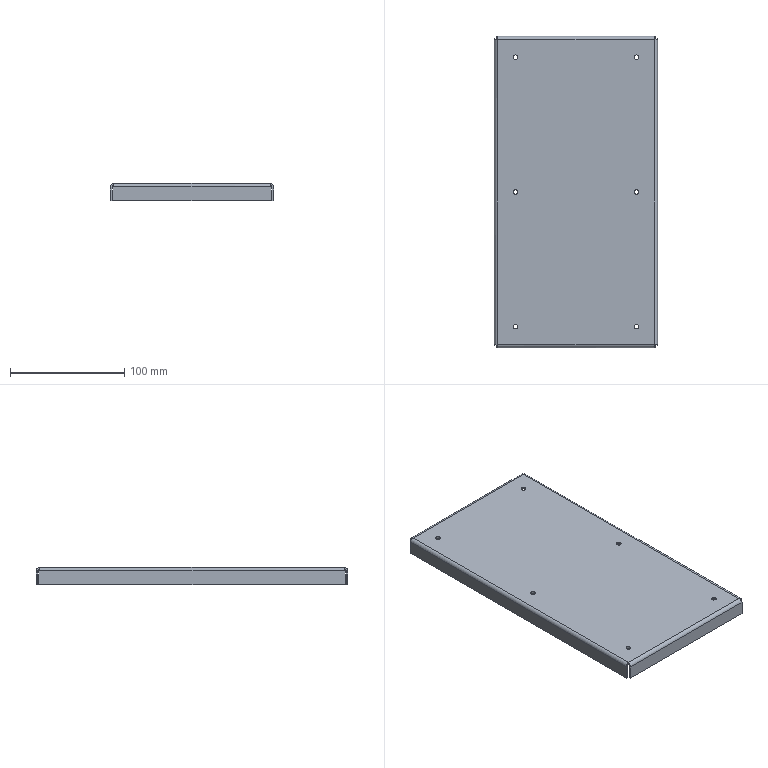Part | STEP file | Driven box door QY-1-38 | 1 solid | 50 faces | box 143 x 273 x 15 mm | volume 73702 mm3 | plane 22 | cylinder 20 | spline 8 | commonest cylinder face diameters 4.2 x12 3 x4 6 x4